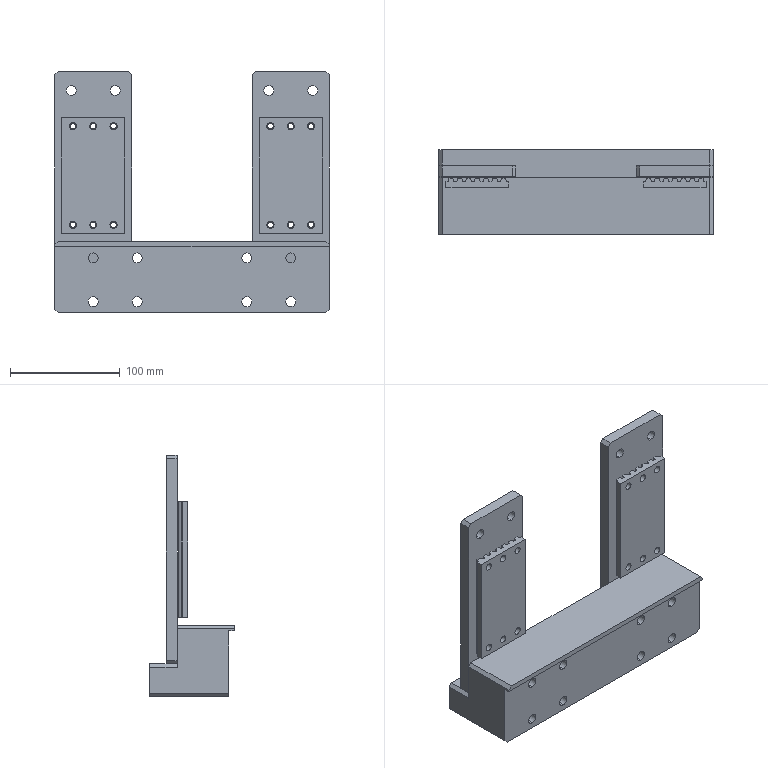Part | SolidWorks | 6 solids | 424 faces | box 250 x 77 x 220 mm | volume 2116355 mm3 | cylinder 260 | plane 120 | cone 44 | commonest cylinder face diameters 9 x48 1.6 x44 10.4 x44 6.8 x32 15 x32 5 x24